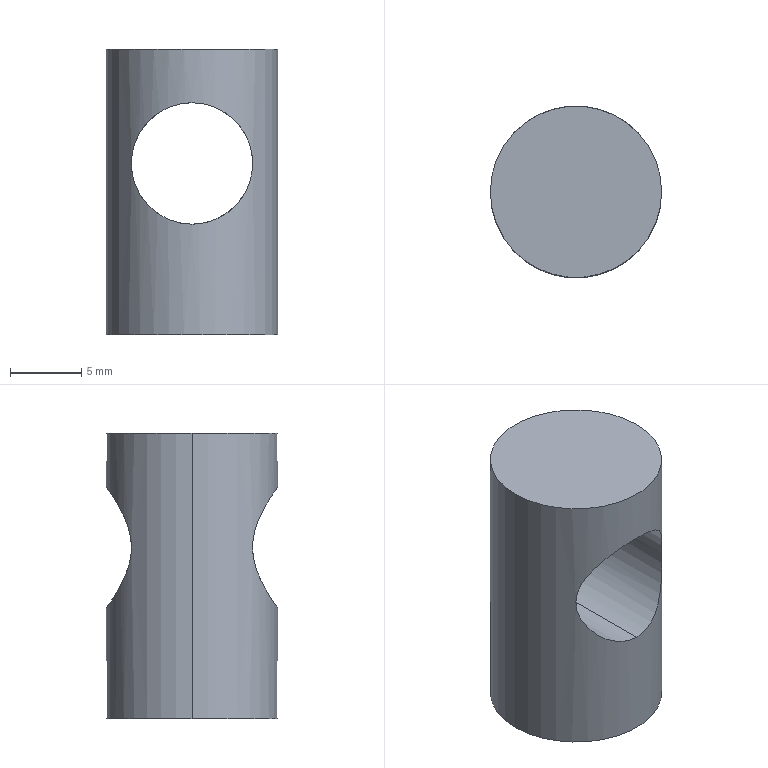Part | SolidWorks | features HoleWzd 2, Extrusion 1 | 1 solid | 6 faces | box 12 x 12 x 20 mm | volume 1627 mm3 | cylinder 4 | plane 2 | commonest cylinder face diameters 8.5 x2 12 x2
STEP:
#1=CARTESIAN_POINT('',(0.,6.,16.25));
#2=VERTEX_POINT('',#1);
#3=CARTESIAN_POINT('',(0.,6.,7.75));
#4=VERTEX_POINT('',#3);
#5=CARTESIAN_POINT('',(0.,6.,16.25));
#6=CARTESIAN_POINT('',(-0.2887,6.,16.25));
#7=CARTESIAN_POINT('',(-0.5762,5.979,16.221));
#8=CARTESIAN_POINT('',(-1.143,5.897,16.104));
#9=CARTESIAN_POINT('',(-1.412,5.838,16.018));
#10=CARTESIAN_POINT('',(-1.928,5.688,15.798));
#11=CARTESIAN_POINT('',(-2.173,5.598,15.663));
#12=CARTESIAN_POINT('',(-2.622,5.402,15.356));
#13=CARTESIAN_POINT('',(-2.831,5.295,15.182));
#14=CARTESIAN_POINT('',(-3.209,5.075,14.8));
#15=CARTESIAN_POINT('',(-3.377,4.963,14.594));
#16=CARTESIAN_POINT('',(-3.676,4.745,14.149));
#17=CARTESIAN_POINT('',(-3.807,4.639,13.908));
#18=CARTESIAN_POINT('',(-4.021,4.455,13.403));
#19=CARTESIAN_POINT('',(-4.105,4.377,13.138));
#20=CARTESIAN_POINT('',(-4.221,4.265,12.575));
#21=CARTESIAN_POINT('',(-4.25,4.235,12.289));
#22=CARTESIAN_POINT('',(-4.25,4.235,11.852));
#23=CARTESIAN_POINT('',(-4.242,4.243,11.705));
#24=CARTESIAN_POINT('',(-4.212,4.273,11.418));
#25=CARTESIAN_POINT('',(-4.191,4.294,11.277));
#26=CARTESIAN_POINT('',(-4.104,4.378,10.86));
#27=CARTESIAN_POINT('',(-4.018,4.458,10.589));
#28=CARTESIAN_POINT('',(-3.697,4.734,9.834));
#29=CARTESIAN_POINT('',(-3.392,4.968,9.384));
#30=CARTESIAN_POINT('',(-2.827,5.297,8.815));
#31=CARTESIAN_POINT('',(-2.617,5.405,8.64));
#32=CARTESIAN_POINT('',(-2.167,5.6,8.334));
#33=CARTESIAN_POINT('',(-1.928,5.688,8.202));
#34=CARTESIAN_POINT('',(-1.417,5.836,7.984));
#35=CARTESIAN_POINT('',(-1.141,5.897,7.896));
#36=CARTESIAN_POINT('',(-0.5799,5.979,7.78));
#37=CARTESIAN_POINT('',(-0.2924,6.,7.75));
#38=CARTESIAN_POINT('',(0.,6.,7.75));
#39=B_SPLINE_CURVE_WITH_KNOTS('',3,(#5,#6,#7,#8,#9,#10,#11,#12,#13,#14,#15,#16,#17,#18,#19,#20,#21,#22,#23,#24,#25,#26,#27,#28,#29,#30,#31,#32,#33,#34,#35,#36,#37,#38),.UNSPECIFIED.,.F.,.F.,(4,2,2,2,2,2,2,2,2,2,2,2,2,2,2,2,4),(0.01383,0.01469,0.01555,0.01642,0.01728,0.01814,0.01901,0.01987,0.02073,0.02116,0.0216,0.02246,0.02418,0.02505,0.02591,0.02677,0.02764),.UNSPECIFIED.);
#40=EDGE_CURVE('',#2,#4,#39,.T.);
#41=ORIENTED_EDGE('',*,*,#40,.F.);
#42=CARTESIAN_POINT('',(0.,-6.,16.25));
#43=VERTEX_POINT('',#42);
#44=CARTESIAN_POINT('',(0.,0.,16.25));
#45=DIRECTION('',(0.,-1.,0.));
#46=VECTOR('',#45,1000.);
#47=LINE('',#44,#46);
#48=EDGE_CURVE('',#2,#43,#47,.T.);
#49=ORIENTED_EDGE('',*,*,#48,.T.);
#50=CARTESIAN_POINT('',(0.,-6.,7.75));
#51=VERTEX_POINT('',#50);
#52=CARTESIAN_POINT('',(0.,-6.,7.75));
#53=CARTESIAN_POINT('',(-0.2887,-6.,7.75));
#54=CARTESIAN_POINT('',(-0.5762,-5.979,7.779));
#55=CARTESIAN_POINT('',(-1.143,-5.897,7.896));
#56=CARTESIAN_POINT('',(-1.412,-5.838,7.982));
#57=CARTESIAN_POINT('',(-1.928,-5.688,8.202));
#58=CARTESIAN_POINT('',(-2.173,-5.598,8.337));
#59=CARTESIAN_POINT('',(-2.622,-5.402,8.644));
#60=CARTESIAN_POINT('',(-2.831,-5.295,8.818));
#61=CARTESIAN_POINT('',(-3.209,-5.075,9.2));
#62=CARTESIAN_POINT('',(-3.377,-4.963,9.406));
#63=CARTESIAN_POINT('',(-3.676,-4.745,9.851));
#64=CARTESIAN_POINT('',(-3.807,-4.639,10.092));
#65=CARTESIAN_POINT('',(-4.021,-4.455,10.597));
#66=CARTESIAN_POINT('',(-4.105,-4.377,10.862));
#67=CARTESIAN_POINT('',(-4.221,-4.265,11.425));
#68=CARTESIAN_POINT('',(-4.25,-4.235,11.711));
#69=CARTESIAN_POINT('',(-4.25,-4.235,12.148));
#70=CARTESIAN_POINT('',(-4.242,-4.243,12.295));
#71=CARTESIAN_POINT('',(-4.212,-4.273,12.582));
#72=CARTESIAN_POINT('',(-4.191,-4.294,12.723));
#73=CARTESIAN_POINT('',(-4.104,-4.378,13.14));
#74=CARTESIAN_POINT('',(-4.018,-4.458,13.411));
#75=CARTESIAN_POINT('',(-3.697,-4.734,14.166));
#76=CARTESIAN_POINT('',(-3.392,-4.968,14.616));
#77=CARTESIAN_POINT('',(-2.827,-5.297,15.185));
#78=CARTESIAN_POINT('',(-2.617,-5.405,15.36));
#79=CARTESIAN_POINT('',(-2.167,-5.6,15.666));
#80=CARTESIAN_POINT('',(-1.928,-5.688,15.798));
#81=CARTESIAN_POINT('',(-1.417,-5.836,16.016));
#82=CARTESIAN_POINT('',(-1.141,-5.897,16.104));
#83=CARTESIAN_POINT('',(-0.5799,-5.979,16.22));
#84=CARTESIAN_POINT('',(-0.2924,-6.,16.25));
#85=CARTESIAN_POINT('',(0.,-6.,16.25));
#86=B_SPLINE_CURVE_WITH_KNOTS('',3,(#52,#53,#54,#55,#56,#57,#58,#59,#60,#61,#62,#63,#64,#65,#66,#67,#68,#69,#70,#71,#72,#73,#74,#75,#76,#77,#78,#79,#80,#81,#82,#83,#84,#85),.UNSPECIFIED.,.F.,.F.,(4,2,2,2,2,2,2,2,2,2,2,2,2,2,2,2,4),(0.01383,0.01469,0.01555,0.01642,0.01728,0.01814,0.01901,0.01987,0.02073,0.02116,0.0216,0.02246,0.02418,0.02505,0.02591,0.02677,0.02764),.UNSPECIFIED.);
#87=EDGE_CURVE('',#51,#43,#86,.T.);
#88=ORIENTED_EDGE('',*,*,#87,.F.);
#89=CARTESIAN_POINT('',(0.,0.,7.75));
#90=DIRECTION('',(0.,-1.,0.));
#91=VECTOR('',#90,1000.);
#92=LINE('',#89,#91);
#93=EDGE_CURVE('',#4,#51,#92,.T.);
#94=ORIENTED_EDGE('',*,*,#93,.F.);
#95=EDGE_LOOP('',(#41,#49,#88,#94));
#96=FACE_OUTER_BOUND('',#95,.T.);
#97=CARTESIAN_POINT('',(0.,0.,12.));
#98=DIRECTION('',(0.,-1.,0.));
#99=DIRECTION('',(0.,0.,-1.));
#100=AXIS2_PLACEMENT_3D('',#97,#98,#99);
#101=CYLINDRICAL_SURFACE('',#100,4.25);
#102=ADVANCED_FACE('',(#96),#101,.F.);
#103=CARTESIAN_POINT('',(0.,6.,7.75));
#104=CARTESIAN_POINT('',(0.2928,6.,7.75));
#105=CARTESIAN_POINT('',(0.579,5.979,7.78));
#106=CARTESIAN_POINT('',(1.139,5.898,7.895));
#107=CARTESIAN_POINT('',(1.415,5.837,7.983));
#108=CARTESIAN_POINT('',(1.928,5.688,8.202));
#109=CARTESIAN_POINT('',(2.171,5.599,8.336));
#110=CARTESIAN_POINT('',(2.624,5.402,8.645));
#111=CARTESIAN_POINT('',(2.83,5.295,8.818));
#112=CARTESIAN_POINT('',(3.207,5.076,9.198));
#113=CARTESIAN_POINT('',(3.379,4.962,9.408));
#114=CARTESIAN_POINT('',(3.677,4.745,9.852));
#115=CARTESIAN_POINT('',(3.805,4.641,10.088));
#116=CARTESIAN_POINT('',(4.02,4.457,10.593));
#117=CARTESIAN_POINT('',(4.105,4.377,10.864));
#118=CARTESIAN_POINT('',(4.191,4.294,11.281));
#119=CARTESIAN_POINT('',(4.213,4.272,11.423));
#120=CARTESIAN_POINT('',(4.243,4.243,11.711));
#121=CARTESIAN_POINT('',(4.25,4.235,11.858));
#122=CARTESIAN_POINT('',(4.25,4.235,12.292));
#123=CARTESIAN_POINT('',(4.22,4.266,12.58));
#124=CARTESIAN_POINT('',(4.104,4.378,13.141));
#125=CARTESIAN_POINT('',(4.02,4.456,13.406));
#126=CARTESIAN_POINT('',(3.806,4.641,13.912));
#127=CARTESIAN_POINT('',(3.674,4.747,14.153));
#128=CARTESIAN_POINT('',(3.376,4.964,14.596));
#129=CARTESIAN_POINT('',(3.207,5.076,14.802));
#130=CARTESIAN_POINT('',(2.829,5.296,15.183));
#131=CARTESIAN_POINT('',(2.62,5.403,15.357));
#132=CARTESIAN_POINT('',(2.173,5.598,15.662));
#133=CARTESIAN_POINT('',(1.933,5.686,15.795));
#134=CARTESIAN_POINT('',(1.416,5.837,16.017));
#135=CARTESIAN_POINT('',(1.143,5.897,16.103));
#136=CARTESIAN_POINT('',(0.5829,5.978,16.22));
#137=CARTESIAN_POINT('',(0.2891,6.,16.25));
#138=CARTESIAN_POINT('',(0.,6.,16.25));
#139=B_SPLINE_CURVE_WITH_KNOTS('',3,(#103,#104,#105,#106,#107,#108,#109,#110,#111,#112,#113,#114,#115,#116,#117,#118,#119,#120,#121,#122,#123,#124,#125,#126,#127,#128,#129,#130,#131,#132,#133,#134,#135,#136,#137,#138),.UNSPECIFIED.,.F.,.F.,(4,2,2,2,2,2,2,2,2,2,2,2,2,2,2,2,2,4),(0.,0.0008643,0.001729,0.002593,0.003457,0.004322,0.005186,0.00605,0.006482,0.006914,0.007779,0.008643,0.009507,0.01037,0.01124,0.0121,0.01296,0.01383),.UNSPECIFIED.);
#140=EDGE_CURVE('',#4,#2,#139,.T.);
#141=ORIENTED_EDGE('',*,*,#140,.T.);
#142=ORIENTED_EDGE('',*,*,#40,.T.);
#143=EDGE_LOOP('',(#141,#142));
#144=FACE_BOUND('',#143,.T.);
#145=CARTESIAN_POINT('',(6.,0.,20.));
#146=VERTEX_POINT('',#145);
#147=CARTESIAN_POINT('',(-6.,0.,20.));
#148=VERTEX_POINT('',#147);
#149=CARTESIAN_POINT('',(0.,0.,20.));
#150=DIRECTION('',(0.,0.,1.));
#151=DIRECTION('',(1.,0.,0.));
#152=AXIS2_PLACEMENT_3D('',#149,#150,#151);
#153=CIRCLE('',#152,6.);
#154=EDGE_CURVE('',#146,#148,#153,.T.);
#155=ORIENTED_EDGE('',*,*,#154,.F.);
#156=CARTESIAN_POINT('',(6.,0.,0.));
#157=VERTEX_POINT('',#156);
#158=CARTESIAN_POINT('',(6.,0.,20.));
#159=DIRECTION('',(0.,0.,-1.));
#160=VECTOR('',#159,1000.);
#161=LINE('',#158,#160);
#162=EDGE_CURVE('',#146,#157,#161,.T.);
#163=ORIENTED_EDGE('',*,*,#162,.T.);
#164=CARTESIAN_POINT('',(-6.,0.,0.));
#165=VERTEX_POINT('',#164);
#166=CARTESIAN_POINT('',(0.,0.,0.));
#167=DIRECTION('',(0.,0.,1.));
#168=DIRECTION('',(1.,0.,0.));
#169=AXIS2_PLACEMENT_3D('',#166,#167,#168);
#170=CIRCLE('',#169,6.);
#171=EDGE_CURVE('',#157,#165,#170,.T.);
#172=ORIENTED_EDGE('',*,*,#171,.T.);
#173=CARTESIAN_POINT('',(-6.,0.,20.));
#174=DIRECTION('',(0.,0.,-1.));
#175=VECTOR('',#174,1000.);
#176=LINE('',#173,#175);
#177=EDGE_CURVE('',#148,#165,#176,.T.);
#178=ORIENTED_EDGE('',*,*,#177,.F.);
#179=EDGE_LOOP('',(#155,#163,#172,#178));
#180=FACE_OUTER_BOUND('',#179,.T.);
#181=CARTESIAN_POINT('',(0.,0.,20.));
#182=DIRECTION('',(0.,0.,-1.));
#183=DIRECTION('',(-1.,0.,0.));
#184=AXIS2_PLACEMENT_3D('',#181,#182,#183);
#185=CYLINDRICAL_SURFACE('',#184,6.);
#186=ADVANCED_FACE('',(#144,#180),#185,.T.);
#187=ORIENTED_EDGE('',*,*,#162,.F.);
#188=CARTESIAN_POINT('',(0.,0.,20.));
#189=DIRECTION('',(0.,0.,1.));
#190=DIRECTION('',(1.,0.,0.));
#191=AXIS2_PLACEMENT_3D('',#188,#189,#190);
#192=CIRCLE('',#191,6.);
#193=EDGE_CURVE('',#148,#146,#192,.T.);
#194=ORIENTED_EDGE('',*,*,#193,.F.);
#195=ORIENTED_EDGE('',*,*,#177,.T.);
#196=CARTESIAN_POINT('',(0.,0.,0.));
#197=DIRECTION('',(0.,0.,1.));
#198=DIRECTION('',(1.,0.,0.));
#199=AXIS2_PLACEMENT_3D('',#196,#197,#198);
#200=CIRCLE('',#199,6.);
#201=EDGE_CURVE('',#165,#157,#200,.T.);
#202=ORIENTED_EDGE('',*,*,#201,.T.);
#203=EDGE_LOOP('',(#187,#194,#195,#202));
#204=FACE_OUTER_BOUND('',#203,.T.);
#205=ORIENTED_EDGE('',*,*,#87,.T.);
#206=CARTESIAN_POINT('',(0.,-6.,16.25));
#207=CARTESIAN_POINT('',(0.2928,-6.,16.25));
#208=CARTESIAN_POINT('',(0.579,-5.979,16.22));
#209=CARTESIAN_POINT('',(1.139,-5.898,16.105));
#210=CARTESIAN_POINT('',(1.415,-5.837,16.017));
#211=CARTESIAN_POINT('',(1.928,-5.688,15.798));
#212=CARTESIAN_POINT('',(2.171,-5.599,15.664));
#213=CARTESIAN_POINT('',(2.624,-5.402,15.355));
#214=CARTESIAN_POINT('',(2.83,-5.295,15.182));
#215=CARTESIAN_POINT('',(3.207,-5.076,14.802));
#216=CARTESIAN_POINT('',(3.379,-4.962,14.592));
#217=CARTESIAN_POINT('',(3.677,-4.745,14.148));
#218=CARTESIAN_POINT('',(3.805,-4.641,13.912));
#219=CARTESIAN_POINT('',(4.02,-4.457,13.407));
#220=CARTESIAN_POINT('',(4.105,-4.377,13.136));
#221=CARTESIAN_POINT('',(4.191,-4.294,12.719));
#222=CARTESIAN_POINT('',(4.213,-4.272,12.577));
#223=CARTESIAN_POINT('',(4.243,-4.243,12.289));
#224=CARTESIAN_POINT('',(4.25,-4.235,12.142));
#225=CARTESIAN_POINT('',(4.25,-4.235,11.708));
#226=CARTESIAN_POINT('',(4.22,-4.266,11.42));
#227=CARTESIAN_POINT('',(4.104,-4.378,10.859));
#228=CARTESIAN_POINT('',(4.02,-4.456,10.594));
#229=CARTESIAN_POINT('',(3.806,-4.641,10.088));
#230=CARTESIAN_POINT('',(3.674,-4.747,9.847));
#231=CARTESIAN_POINT('',(3.376,-4.964,9.404));
#232=CARTESIAN_POINT('',(3.207,-5.076,9.198));
#233=CARTESIAN_POINT('',(2.829,-5.296,8.817));
#234=CARTESIAN_POINT('',(2.62,-5.403,8.643));
#235=CARTESIAN_POINT('',(2.173,-5.598,8.338));
#236=CARTESIAN_POINT('',(1.933,-5.686,8.205));
#237=CARTESIAN_POINT('',(1.416,-5.837,7.983));
#238=CARTESIAN_POINT('',(1.143,-5.897,7.897));
#239=CARTESIAN_POINT('',(0.5829,-5.978,7.78));
#240=CARTESIAN_POINT('',(0.2891,-6.,7.75));
#241=CARTESIAN_POINT('',(0.,-6.,7.75));
#242=B_SPLINE_CURVE_WITH_KNOTS('',3,(#206,#207,#208,#209,#210,#211,#212,#213,#214,#215,#216,#217,#218,#219,#220,#221,#222,#223,#224,#225,#226,#227,#228,#229,#230,#231,#232,#233,#234,#235,#236,#237,#238,#239,#240,#241),.UNSPECIFIED.,.F.,.F.,(4,2,2,2,2,2,2,2,2,2,2,2,2,2,2,2,2,4),(0.,0.0008643,0.001729,0.002593,0.003457,0.004322,0.005186,0.00605,0.006482,0.006914,0.007779,0.008643,0.009507,0.01037,0.01124,0.0121,0.01296,0.01383),.UNSPECIFIED.);
#243=EDGE_CURVE('',#43,#51,#242,.T.);
#244=ORIENTED_EDGE('',*,*,#243,.T.);
#245=EDGE_LOOP('',(#205,#244));
#246=FACE_BOUND('',#245,.T.);
#247=CARTESIAN_POINT('',(0.,0.,20.));
#248=DIRECTION('',(0.,0.,-1.));
#249=DIRECTION('',(-1.,0.,0.));
#250=AXIS2_PLACEMENT_3D('',#247,#248,#249);
#251=CYLINDRICAL_SURFACE('',#250,6.);
#252=ADVANCED_FACE('',(#204,#246),#251,.T.);
#253=ORIENTED_EDGE('',*,*,#193,.T.);
#254=ORIENTED_EDGE('',*,*,#154,.T.);
#255=EDGE_LOOP('',(#253,#254));
#256=FACE_OUTER_BOUND('',#255,.T.);
#257=CARTESIAN_POINT('',(0.,0.,20.));
#258=DIRECTION('',(0.,0.,1.));
#259=DIRECTION('',(1.,0.,0.));
#260=AXIS2_PLACEMENT_3D('',#257,#258,#259);
#261=PLANE('',#260);
#262=ADVANCED_FACE('',(#256),#261,.T.);
#263=ORIENTED_EDGE('',*,*,#201,.F.);
#264=ORIENTED_EDGE('',*,*,#171,.F.);
#265=EDGE_LOOP('',(#263,#264));
#266=FACE_OUTER_BOUND('',#265,.T.);
#267=CARTESIAN_POINT('',(0.,0.,0.));
#268=DIRECTION('',(0.,0.,1.));
#269=DIRECTION('',(1.,0.,0.));
#270=AXIS2_PLACEMENT_3D('',#267,#268,#269);
#271=PLANE('',#270);
#272=ADVANCED_FACE('',(#266),#271,.F.);
#273=ORIENTED_EDGE('',*,*,#48,.F.);
#274=ORIENTED_EDGE('',*,*,#140,.F.);
#275=ORIENTED_EDGE('',*,*,#93,.T.);
#276=ORIENTED_EDGE('',*,*,#243,.F.);
#277=EDGE_LOOP('',(#273,#274,#275,#276));
#278=FACE_OUTER_BOUND('',#277,.T.);
#279=CARTESIAN_POINT('',(0.,0.,12.));
#280=DIRECTION('',(0.,-1.,0.));
#281=DIRECTION('',(0.,0.,-1.));
#282=AXIS2_PLACEMENT_3D('',#279,#280,#281);
#283=CYLINDRICAL_SURFACE('',#282,4.25);
#284=ADVANCED_FACE('',(#278),#283,.F.);
#285=CLOSED_SHELL('',(#102,#186,#252,#262,#272,#284));
#286=MANIFOLD_SOLID_BREP('',#285);
#287=CARTESIAN_POINT('',(0.,0.,0.));
#288=DIRECTION('',(0.,0.,1.));
#289=DIRECTION('',(1.,0.,0.));
#290=AXIS2_PLACEMENT_3D('',#287,#288,#289);
#291=(LENGTH_UNIT()NAMED_UNIT(*)SI_UNIT(.MILLI.,.METRE.));
#292=UNCERTAINTY_MEASURE_WITH_UNIT(LENGTH_MEASURE(0.00001),#291,'','');
#293=(NAMED_UNIT(*)PLANE_ANGLE_UNIT()SI_UNIT($,.RADIAN.));
#294=(NAMED_UNIT(*)SI_UNIT($,.STERADIAN.)SOLID_ANGLE_UNIT());
#295=(GEOMETRIC_REPRESENTATION_CONTEXT(3)GLOBAL_UNCERTAINTY_ASSIGNED_CONTEXT((#292))GLOBAL_UNIT_ASSIGNED_CONTEXT((#291,#293,#294))REPRESENTATION_CONTEXT('',''));
#296=ADVANCED_BREP_SHAPE_REPRESENTATION('',(#286,#290),#295);